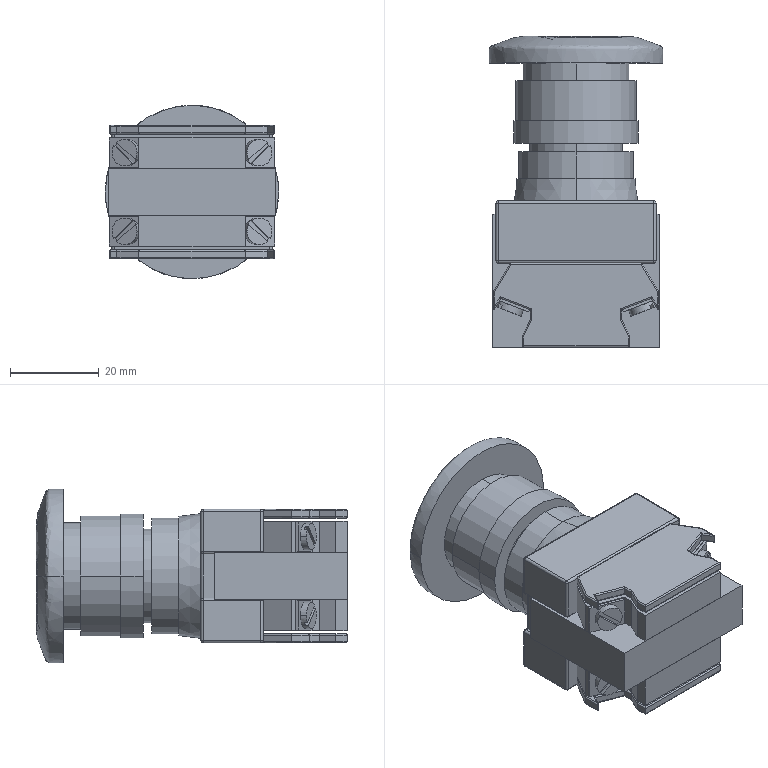Part | SolidWorks | features BaseBody 3 | 3 solids | 317 faces | box 39 x 70 x 39 mm | volume 55786 mm3 | plane 152 | cylinder 132 | spline 31 | cone 2 | commonest cylinder face diameters 0.6 x64 1 x34 6 x8 0.24 x4 24.115 x4 28.112 x4